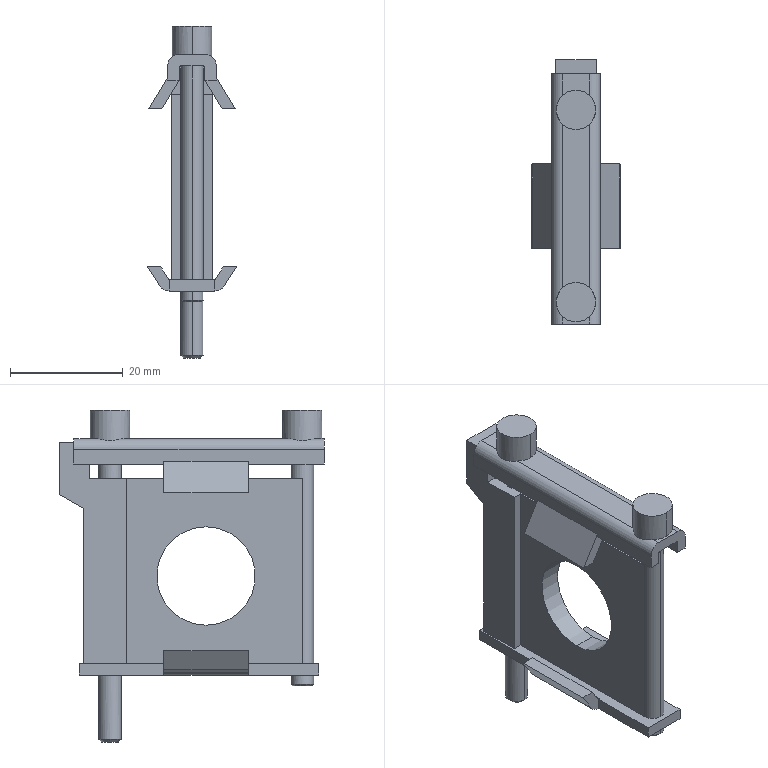Part | NX | 1 solid | 96 faces | box 15.9 x 47 x 59 mm | volume 8626 mm3 | plane 70 | cylinder 22 | cone 4 | commonest cylinder face diameters 4 x10 7 x4 0.6 x2 1 x2 3.8 x2 17.5 x2